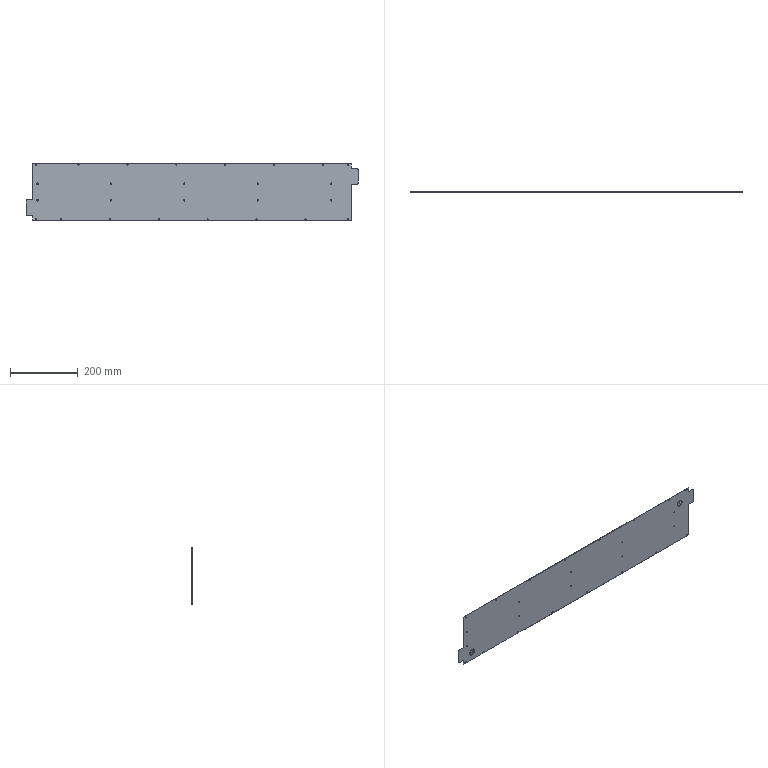Part | NX | features BREP 1 | 1 solid | 104 faces | box 983.7 x 0.7 x 171.2 mm | volume 81617 mm3 | cylinder 68 | plane 36 | commonest cylinder face diameters 3.8 x52 4 x4 6 x4 16 x4 20 x4